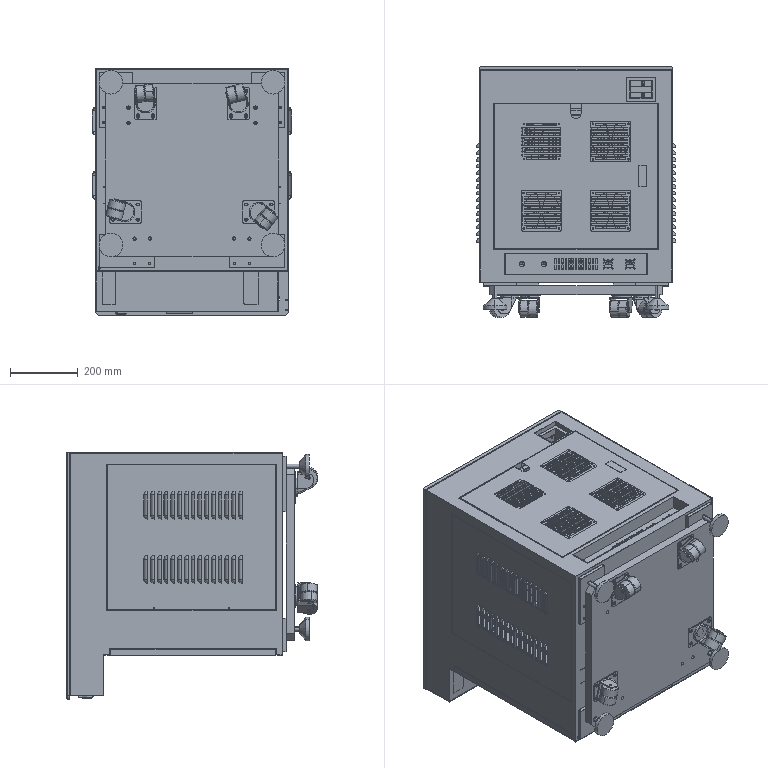Part | SolidWorks | 47 solids | 5764 faces | volume 2228095 mm3 | cylinder 2875 | plane 2157 | sphere 300 | spline 292 | cone 108 | torus 32 | commonest cylinder face diameters 4.2 x395 5 x366 6 x233 3 x208 3.2 x164 20 x149